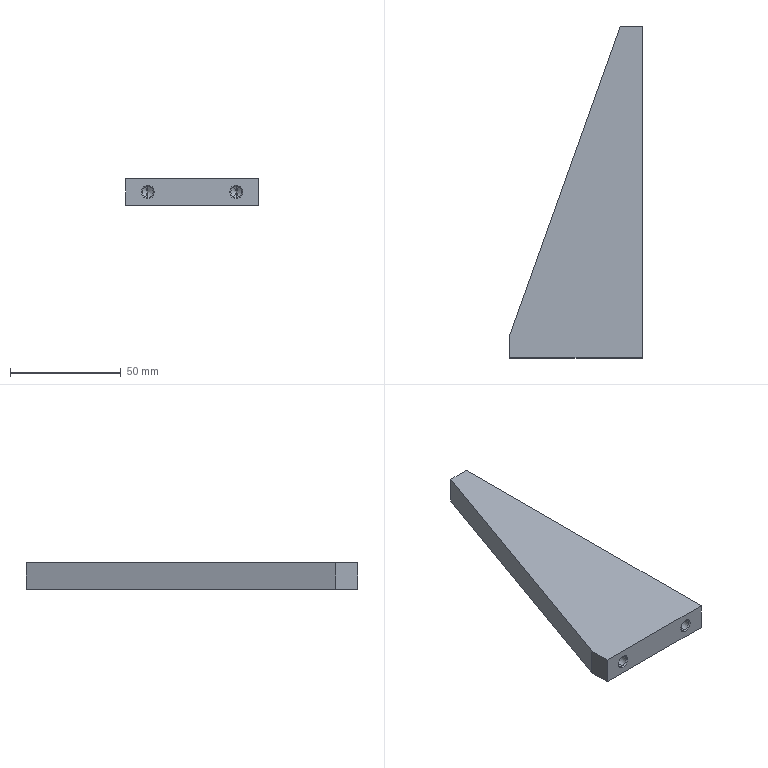Part | SolidWorks | features HoleWzd 2, Extrusion 1 | 1 solid | 31 faces | box 60 x 150 x 12 mm | volume 64773 mm3 | cone 16 | cylinder 8 | plane 7 | commonest cylinder face diameters 5 x8
STEP:
#1=CARTESIAN_POINT('',(59.475,33.456,8.5));
#2=VERTEX_POINT('',#1);
#3=CARTESIAN_POINT('',(59.475,33.456,3.5));
#4=VERTEX_POINT('',#3);
#5=CARTESIAN_POINT('',(59.475,33.456,6.));
#6=DIRECTION('',(1.,0.,0.));
#7=DIRECTION('',(0.,0.,-1.));
#8=AXIS2_PLACEMENT_3D('',#5,#6,#7);
#9=CIRCLE('',#8,2.5);
#10=EDGE_CURVE('',#2,#4,#9,.T.);
#11=ORIENTED_EDGE('',*,*,#10,.F.);
#12=CARTESIAN_POINT('',(60.,33.456,9.025));
#13=VERTEX_POINT('',#12);
#14=CARTESIAN_POINT('',(60.,33.456,9.025));
#15=DIRECTION('',(0.7071,0.,0.7071));
#16=VECTOR('',#15,1000.);
#17=LINE('',#14,#16);
#18=EDGE_CURVE('',#2,#13,#17,.T.);
#19=ORIENTED_EDGE('',*,*,#18,.T.);
#20=CARTESIAN_POINT('',(60.,33.456,2.975));
#21=VERTEX_POINT('',#20);
#22=CARTESIAN_POINT('',(60.,33.456,6.));
#23=DIRECTION('',(1.,0.,0.));
#24=DIRECTION('',(0.,0.,-1.));
#25=AXIS2_PLACEMENT_3D('',#22,#23,#24);
#26=CIRCLE('',#25,3.025);
#27=EDGE_CURVE('',#13,#21,#26,.T.);
#28=ORIENTED_EDGE('',*,*,#27,.T.);
#29=CARTESIAN_POINT('',(60.,33.456,2.975));
#30=DIRECTION('',(0.7071,0.,-0.7071));
#31=VECTOR('',#30,1000.);
#32=LINE('',#29,#31);
#33=EDGE_CURVE('',#4,#21,#32,.T.);
#34=ORIENTED_EDGE('',*,*,#33,.F.);
#35=EDGE_LOOP('',(#11,#19,#28,#34));
#36=FACE_OUTER_BOUND('',#35,.T.);
#37=CARTESIAN_POINT('',(60.,33.456,6.));
#38=DIRECTION('',(1.,0.,0.));
#39=DIRECTION('',(0.,0.,-1.));
#40=AXIS2_PLACEMENT_3D('',#37,#38,#39);
#41=CONICAL_SURFACE('',#40,3.025,0.7854);
#42=ADVANCED_FACE('',(#36),#41,.F.);
#43=CARTESIAN_POINT('',(45.,33.456,8.5));
#44=VERTEX_POINT('',#43);
#45=CARTESIAN_POINT('',(45.,33.456,3.5));
#46=VERTEX_POINT('',#45);
#47=CARTESIAN_POINT('',(45.,33.456,6.));
#48=DIRECTION('',(1.,0.,0.));
#49=DIRECTION('',(0.,0.,-1.));
#50=AXIS2_PLACEMENT_3D('',#47,#48,#49);
#51=CIRCLE('',#50,2.5);
#52=EDGE_CURVE('',#44,#46,#51,.T.);
#53=ORIENTED_EDGE('',*,*,#52,.F.);
#54=CARTESIAN_POINT('',(60.,33.456,8.5));
#55=DIRECTION('',(1.,0.,0.));
#56=VECTOR('',#55,1000.);
#57=LINE('',#54,#56);
#58=EDGE_CURVE('',#44,#2,#57,.T.);
#59=ORIENTED_EDGE('',*,*,#58,.T.);
#60=ORIENTED_EDGE('',*,*,#10,.T.);
#61=CARTESIAN_POINT('',(60.,33.456,3.5));
#62=DIRECTION('',(1.,0.,0.));
#63=VECTOR('',#62,1000.);
#64=LINE('',#61,#63);
#65=EDGE_CURVE('',#46,#4,#64,.T.);
#66=ORIENTED_EDGE('',*,*,#65,.F.);
#67=EDGE_LOOP('',(#53,#59,#60,#66));
#68=FACE_OUTER_BOUND('',#67,.T.);
#69=CARTESIAN_POINT('',(60.,33.456,6.));
#70=DIRECTION('',(1.,0.,0.));
#71=DIRECTION('',(0.,0.,-1.));
#72=AXIS2_PLACEMENT_3D('',#69,#70,#71);
#73=CYLINDRICAL_SURFACE('',#72,2.5);
#74=ADVANCED_FACE('',(#68),#73,.F.);
#75=CARTESIAN_POINT('',(43.498,33.456,6.));
#76=VERTEX_POINT('',#75);
#77=CARTESIAN_POINT('',(45.,33.456,3.5));
#78=DIRECTION('',(0.515,0.,-0.8572));
#79=VECTOR('',#78,1000.);
#80=LINE('',#77,#79);
#81=EDGE_CURVE('',#76,#46,#80,.T.);
#82=ORIENTED_EDGE('',*,*,#81,.F.);
#83=CARTESIAN_POINT('',(45.,33.456,8.5));
#84=DIRECTION('',(0.515,0.,0.8572));
#85=VECTOR('',#84,1000.);
#86=LINE('',#83,#85);
#87=EDGE_CURVE('',#76,#44,#86,.T.);
#88=ORIENTED_EDGE('',*,*,#87,.T.);
#89=ORIENTED_EDGE('',*,*,#52,.T.);
#90=EDGE_LOOP('',(#82,#88,#89));
#91=FACE_OUTER_BOUND('',#90,.T.);
#92=CARTESIAN_POINT('',(45.,33.456,6.));
#93=DIRECTION('',(1.,0.,0.));
#94=DIRECTION('',(0.,0.,-1.));
#95=AXIS2_PLACEMENT_3D('',#92,#93,#94);
#96=CONICAL_SURFACE('',#95,2.5,1.03);
#97=ADVANCED_FACE('',(#91),#96,.F.);
#98=CARTESIAN_POINT('',(59.475,133.456,8.5));
#99=VERTEX_POINT('',#98);
#100=CARTESIAN_POINT('',(59.475,133.456,3.5));
#101=VERTEX_POINT('',#100);
#102=CARTESIAN_POINT('',(59.475,133.456,6.));
#103=DIRECTION('',(1.,0.,0.));
#104=DIRECTION('',(0.,0.,-1.));
#105=AXIS2_PLACEMENT_3D('',#102,#103,#104);
#106=CIRCLE('',#105,2.5);
#107=EDGE_CURVE('',#99,#101,#106,.T.);
#108=ORIENTED_EDGE('',*,*,#107,.F.);
#109=CARTESIAN_POINT('',(60.,133.456,9.025));
#110=VERTEX_POINT('',#109);
#111=CARTESIAN_POINT('',(60.,133.456,9.025));
#112=DIRECTION('',(0.7071,0.,0.7071));
#113=VECTOR('',#112,1000.);
#114=LINE('',#111,#113);
#115=EDGE_CURVE('',#99,#110,#114,.T.);
#116=ORIENTED_EDGE('',*,*,#115,.T.);
#117=CARTESIAN_POINT('',(60.,133.456,2.975));
#118=VERTEX_POINT('',#117);
#119=CARTESIAN_POINT('',(60.,133.456,6.));
#120=DIRECTION('',(1.,0.,0.));
#121=DIRECTION('',(0.,0.,-1.));
#122=AXIS2_PLACEMENT_3D('',#119,#120,#121);
#123=CIRCLE('',#122,3.025);
#124=EDGE_CURVE('',#110,#118,#123,.T.);
#125=ORIENTED_EDGE('',*,*,#124,.T.);
#126=CARTESIAN_POINT('',(60.,133.456,2.975));
#127=DIRECTION('',(0.7071,0.,-0.7071));
#128=VECTOR('',#127,1000.);
#129=LINE('',#126,#128);
#130=EDGE_CURVE('',#101,#118,#129,.T.);
#131=ORIENTED_EDGE('',*,*,#130,.F.);
#132=EDGE_LOOP('',(#108,#116,#125,#131));
#133=FACE_OUTER_BOUND('',#132,.T.);
#134=CARTESIAN_POINT('',(60.,133.456,6.));
#135=DIRECTION('',(1.,0.,0.));
#136=DIRECTION('',(0.,0.,-1.));
#137=AXIS2_PLACEMENT_3D('',#134,#135,#136);
#138=CONICAL_SURFACE('',#137,3.025,0.7854);
#139=ADVANCED_FACE('',(#133),#138,.F.);
#140=CARTESIAN_POINT('',(45.,133.456,8.5));
#141=VERTEX_POINT('',#140);
#142=CARTESIAN_POINT('',(45.,133.456,3.5));
#143=VERTEX_POINT('',#142);
#144=CARTESIAN_POINT('',(45.,133.456,6.));
#145=DIRECTION('',(1.,0.,0.));
#146=DIRECTION('',(0.,0.,-1.));
#147=AXIS2_PLACEMENT_3D('',#144,#145,#146);
#148=CIRCLE('',#147,2.5);
#149=EDGE_CURVE('',#141,#143,#148,.T.);
#150=ORIENTED_EDGE('',*,*,#149,.F.);
#151=CARTESIAN_POINT('',(60.,133.456,8.5));
#152=DIRECTION('',(1.,0.,0.));
#153=VECTOR('',#152,1000.);
#154=LINE('',#151,#153);
#155=EDGE_CURVE('',#141,#99,#154,.T.);
#156=ORIENTED_EDGE('',*,*,#155,.T.);
#157=ORIENTED_EDGE('',*,*,#107,.T.);
#158=CARTESIAN_POINT('',(60.,133.456,3.5));
#159=DIRECTION('',(1.,0.,0.));
#160=VECTOR('',#159,1000.);
#161=LINE('',#158,#160);
#162=EDGE_CURVE('',#143,#101,#161,.T.);
#163=ORIENTED_EDGE('',*,*,#162,.F.);
#164=EDGE_LOOP('',(#150,#156,#157,#163));
#165=FACE_OUTER_BOUND('',#164,.T.);
#166=CARTESIAN_POINT('',(60.,133.456,6.));
#167=DIRECTION('',(1.,0.,0.));
#168=DIRECTION('',(0.,0.,-1.));
#169=AXIS2_PLACEMENT_3D('',#166,#167,#168);
#170=CYLINDRICAL_SURFACE('',#169,2.5);
#171=ADVANCED_FACE('',(#165),#170,.F.);
#172=CARTESIAN_POINT('',(43.498,133.456,6.));
#173=VERTEX_POINT('',#172);
#174=CARTESIAN_POINT('',(45.,133.456,3.5));
#175=DIRECTION('',(0.515,0.,-0.8572));
#176=VECTOR('',#175,1000.);
#177=LINE('',#174,#176);
#178=EDGE_CURVE('',#173,#143,#177,.T.);
#179=ORIENTED_EDGE('',*,*,#178,.F.);
#180=CARTESIAN_POINT('',(45.,133.456,8.5));
#181=DIRECTION('',(0.515,0.,0.8572));
#182=VECTOR('',#181,1000.);
#183=LINE('',#180,#182);
#184=EDGE_CURVE('',#173,#141,#183,.T.);
#185=ORIENTED_EDGE('',*,*,#184,.T.);
#186=ORIENTED_EDGE('',*,*,#149,.T.);
#187=EDGE_LOOP('',(#179,#185,#186));
#188=FACE_OUTER_BOUND('',#187,.T.);
#189=CARTESIAN_POINT('',(45.,133.456,6.));
#190=DIRECTION('',(1.,0.,0.));
#191=DIRECTION('',(0.,0.,-1.));
#192=AXIS2_PLACEMENT_3D('',#189,#190,#191);
#193=CONICAL_SURFACE('',#192,2.5,1.03);
#194=ADVANCED_FACE('',(#188),#193,.F.);
#195=CARTESIAN_POINT('',(50.,8.981,8.5));
#196=VERTEX_POINT('',#195);
#197=CARTESIAN_POINT('',(50.,8.981,3.5));
#198=VERTEX_POINT('',#197);
#199=CARTESIAN_POINT('',(50.,8.981,6.));
#200=DIRECTION('',(0.,-1.,0.));
#201=DIRECTION('',(0.,0.,-1.));
#202=AXIS2_PLACEMENT_3D('',#199,#200,#201);
#203=CIRCLE('',#202,2.5);
#204=EDGE_CURVE('',#196,#198,#203,.T.);
#205=ORIENTED_EDGE('',*,*,#204,.F.);
#206=CARTESIAN_POINT('',(50.,8.456,9.025));
#207=VERTEX_POINT('',#206);
#208=CARTESIAN_POINT('',(50.,8.456,9.025));
#209=DIRECTION('',(0.,-0.7071,0.7071));
#210=VECTOR('',#209,1000.);
#211=LINE('',#208,#210);
#212=EDGE_CURVE('',#196,#207,#211,.T.);
#213=ORIENTED_EDGE('',*,*,#212,.T.);
#214=CARTESIAN_POINT('',(50.,8.456,2.975));
#215=VERTEX_POINT('',#214);
#216=CARTESIAN_POINT('',(50.,8.456,6.));
#217=DIRECTION('',(0.,-1.,0.));
#218=DIRECTION('',(0.,0.,-1.));
#219=AXIS2_PLACEMENT_3D('',#216,#217,#218);
#220=CIRCLE('',#219,3.025);
#221=EDGE_CURVE('',#207,#215,#220,.T.);
#222=ORIENTED_EDGE('',*,*,#221,.T.);
#223=CARTESIAN_POINT('',(50.,8.456,2.975));
#224=DIRECTION('',(0.,-0.7071,-0.7071));
#225=VECTOR('',#224,1000.);
#226=LINE('',#223,#225);
#227=EDGE_CURVE('',#198,#215,#226,.T.);
#228=ORIENTED_EDGE('',*,*,#227,.F.);
#229=EDGE_LOOP('',(#205,#213,#222,#228));
#230=FACE_OUTER_BOUND('',#229,.T.);
#231=CARTESIAN_POINT('',(50.,8.456,6.));
#232=DIRECTION('',(0.,-1.,0.));
#233=DIRECTION('',(0.,0.,-1.));
#234=AXIS2_PLACEMENT_3D('',#231,#232,#233);
#235=CONICAL_SURFACE('',#234,3.025,0.7854);
#236=ADVANCED_FACE('',(#230),#235,.F.);
#237=CARTESIAN_POINT('',(50.,23.456,8.5));
#238=VERTEX_POINT('',#237);
#239=CARTESIAN_POINT('',(50.,23.456,3.5));
#240=VERTEX_POINT('',#239);
#241=CARTESIAN_POINT('',(50.,23.456,6.));
#242=DIRECTION('',(0.,-1.,0.));
#243=DIRECTION('',(0.,0.,-1.));
#244=AXIS2_PLACEMENT_3D('',#241,#242,#243);
#245=CIRCLE('',#244,2.5);
#246=EDGE_CURVE('',#238,#240,#245,.T.);
#247=ORIENTED_EDGE('',*,*,#246,.F.);
#248=CARTESIAN_POINT('',(50.,8.456,8.5));
#249=DIRECTION('',(0.,-1.,0.));
#250=VECTOR('',#249,1000.);
#251=LINE('',#248,#250);
#252=EDGE_CURVE('',#238,#196,#251,.T.);
#253=ORIENTED_EDGE('',*,*,#252,.T.);
#254=ORIENTED_EDGE('',*,*,#204,.T.);
#255=CARTESIAN_POINT('',(50.,8.456,3.5));
#256=DIRECTION('',(0.,-1.,0.));
#257=VECTOR('',#256,1000.);
#258=LINE('',#255,#257);
#259=EDGE_CURVE('',#240,#198,#258,.T.);
#260=ORIENTED_EDGE('',*,*,#259,.F.);
#261=EDGE_LOOP('',(#247,#253,#254,#260));
#262=FACE_OUTER_BOUND('',#261,.T.);
#263=CARTESIAN_POINT('',(50.,8.456,6.));
#264=DIRECTION('',(0.,-1.,0.));
#265=DIRECTION('',(0.,0.,-1.));
#266=AXIS2_PLACEMENT_3D('',#263,#264,#265);
#267=CYLINDRICAL_SURFACE('',#266,2.5);
#268=ADVANCED_FACE('',(#262),#267,.F.);
#269=CARTESIAN_POINT('',(50.,24.959,6.));
#270=VERTEX_POINT('',#269);
#271=CARTESIAN_POINT('',(50.,23.456,3.5));
#272=DIRECTION('',(0.,-0.515,-0.8572));
#273=VECTOR('',#272,1000.);
#274=LINE('',#271,#273);
#275=EDGE_CURVE('',#270,#240,#274,.T.);
#276=ORIENTED_EDGE('',*,*,#275,.F.);
#277=CARTESIAN_POINT('',(50.,23.456,8.5));
#278=DIRECTION('',(0.,-0.515,0.8572));
#279=VECTOR('',#278,1000.);
#280=LINE('',#277,#279);
#281=EDGE_CURVE('',#270,#238,#280,.T.);
#282=ORIENTED_EDGE('',*,*,#281,.T.);
#283=ORIENTED_EDGE('',*,*,#246,.T.);
#284=EDGE_LOOP('',(#276,#282,#283));
#285=FACE_OUTER_BOUND('',#284,.T.);
#286=CARTESIAN_POINT('',(50.,23.456,6.));
#287=DIRECTION('',(0.,-1.,0.));
#288=DIRECTION('',(0.,0.,-1.));
#289=AXIS2_PLACEMENT_3D('',#286,#287,#288);
#290=CONICAL_SURFACE('',#289,2.5,1.03);
#291=ADVANCED_FACE('',(#285),#290,.F.);
#292=CARTESIAN_POINT('',(10.,8.981,8.5));
#293=VERTEX_POINT('',#292);
#294=CARTESIAN_POINT('',(10.,8.981,3.5));
#295=VERTEX_POINT('',#294);
#296=CARTESIAN_POINT('',(10.,8.981,6.));
#297=DIRECTION('',(0.,-1.,0.));
#298=DIRECTION('',(0.,0.,-1.));
#299=AXIS2_PLACEMENT_3D('',#296,#297,#298);
#300=CIRCLE('',#299,2.5);
#301=EDGE_CURVE('',#293,#295,#300,.T.);
#302=ORIENTED_EDGE('',*,*,#301,.F.);
#303=CARTESIAN_POINT('',(10.,8.456,9.025));
#304=VERTEX_POINT('',#303);
#305=CARTESIAN_POINT('',(10.,8.456,9.025));
#306=DIRECTION('',(0.,-0.7071,0.7071));
#307=VECTOR('',#306,1000.);
#308=LINE('',#305,#307);
#309=EDGE_CURVE('',#293,#304,#308,.T.);
#310=ORIENTED_EDGE('',*,*,#309,.T.);
#311=CARTESIAN_POINT('',(10.,8.456,2.975));
#312=VERTEX_POINT('',#311);
#313=CARTESIAN_POINT('',(10.,8.456,6.));
#314=DIRECTION('',(0.,-1.,0.));
#315=DIRECTION('',(0.,0.,-1.));
#316=AXIS2_PLACEMENT_3D('',#313,#314,#315);
#317=CIRCLE('',#316,3.025);
#318=EDGE_CURVE('',#304,#312,#317,.T.);
#319=ORIENTED_EDGE('',*,*,#318,.T.);
#320=CARTESIAN_POINT('',(10.,8.456,2.975));
#321=DIRECTION('',(0.,-0.7071,-0.7071));
#322=VECTOR('',#321,1000.);
#323=LINE('',#320,#322);
#324=EDGE_CURVE('',#295,#312,#323,.T.);
#325=ORIENTED_EDGE('',*,*,#324,.F.);
#326=EDGE_LOOP('',(#302,#310,#319,#325));
#327=FACE_OUTER_BOUND('',#326,.T.);
#328=CARTESIAN_POINT('',(10.,8.456,6.));
#329=DIRECTION('',(0.,-1.,0.));
#330=DIRECTION('',(0.,0.,-1.));
#331=AXIS2_PLACEMENT_3D('',#328,#329,#330);
#332=CONICAL_SURFACE('',#331,3.025,0.7854);
#333=ADVANCED_FACE('',(#327),#332,.F.);
#334=CARTESIAN_POINT('',(10.,23.456,8.5));
#335=VERTEX_POINT('',#334);
#336=CARTESIAN_POINT('',(10.,23.456,3.5));
#337=VERTEX_POINT('',#336);
#338=CARTESIAN_POINT('',(10.,23.456,6.));
#339=DIRECTION('',(0.,-1.,0.));
#340=DIRECTION('',(0.,0.,-1.));
#341=AXIS2_PLACEMENT_3D('',#338,#339,#340);
#342=CIRCLE('',#341,2.5);
#343=EDGE_CURVE('',#335,#337,#342,.T.);
#344=ORIENTED_EDGE('',*,*,#343,.F.);
#345=CARTESIAN_POINT('',(10.,8.456,8.5));
#346=DIRECTION('',(0.,-1.,0.));
#347=VECTOR('',#346,1000.);
#348=LINE('',#345,#347);
#349=EDGE_CURVE('',#335,#293,#348,.T.);
#350=ORIENTED_EDGE('',*,*,#349,.T.);
#351=ORIENTED_EDGE('',*,*,#301,.T.);
#352=CARTESIAN_POINT('',(10.,8.456,3.5));
#353=DIRECTION('',(0.,-1.,0.));
#354=VECTOR('',#353,1000.);
#355=LINE('',#352,#354);
#356=EDGE_CURVE('',#337,#295,#355,.T.);
#357=ORIENTED_EDGE('',*,*,#356,.F.);
#358=EDGE_LOOP('',(#344,#350,#351,#357));
#359=FACE_OUTER_BOUND('',#358,.T.);
#360=CARTESIAN_POINT('',(10.,8.456,6.));
#361=DIRECTION('',(0.,-1.,0.));
#362=DIRECTION('',(0.,0.,-1.));
#363=AXIS2_PLACEMENT_3D('',#360,#361,#362);
#364=CYLINDRICAL_SURFACE('',#363,2.5);
#365=ADVANCED_FACE('',(#359),#364,.F.);
#366=CARTESIAN_POINT('',(10.,24.959,6.));
#367=VERTEX_POINT('',#366);
#368=CARTESIAN_POINT('',(10.,23.456,3.5));
#369=DIRECTION('',(0.,-0.515,-0.8572));
#370=VECTOR('',#369,1000.);
#371=LINE('',#368,#370);
#372=EDGE_CURVE('',#367,#337,#371,.T.);
#373=ORIENTED_EDGE('',*,*,#372,.F.);
#374=CARTESIAN_POINT('',(10.,23.456,8.5));
#375=DIRECTION('',(0.,-0.515,0.8572));
#376=VECTOR('',#375,1000.);
#377=LINE('',#374,#376);
#378=EDGE_CURVE('',#367,#335,#377,.T.);
#379=ORIENTED_EDGE('',*,*,#378,.T.);
#380=ORIENTED_EDGE('',*,*,#343,.T.);
#381=EDGE_LOOP('',(#373,#379,#380));
#382=FACE_OUTER_BOUND('',#381,.T.);
#383=CARTESIAN_POINT('',(10.,23.456,6.));
#384=DIRECTION('',(0.,-1.,0.));
#385=DIRECTION('',(0.,0.,-1.));
#386=AXIS2_PLACEMENT_3D('',#383,#384,#385);
#387=CONICAL_SURFACE('',#386,2.5,1.03);
#388=ADVANCED_FACE('',(#382),#387,.F.);
#389=CARTESIAN_POINT('',(50.,158.456,0.));
#390=VERTEX_POINT('',#389);
#391=CARTESIAN_POINT('',(0.,18.456,0.));
#392=VERTEX_POINT('',#391);
#393=CARTESIAN_POINT('',(0.,18.456,0.));
#394=DIRECTION('',(-0.3363,-0.9417,0.));
#395=VECTOR('',#394,1000.);
#396=LINE('',#393,#395);
#397=EDGE_CURVE('',#390,#392,#396,.T.);
#398=ORIENTED_EDGE('',*,*,#397,.T.);
#399=CARTESIAN_POINT('',(0.,18.456,12.));
#400=VERTEX_POINT('',#399);
#401=CARTESIAN_POINT('',(0.,18.456,12.));
#402=DIRECTION('',(0.,0.,-1.));
#403=VECTOR('',#402,1000.);
#404=LINE('',#401,#403);
#405=EDGE_CURVE('',#400,#392,#404,.T.);
#406=ORIENTED_EDGE('',*,*,#405,.F.);
#407=CARTESIAN_POINT('',(50.,158.456,12.));
#408=VERTEX_POINT('',#407);
#409=CARTESIAN_POINT('',(0.,18.456,12.));
#410=DIRECTION('',(-0.3363,-0.9417,0.));
#411=VECTOR('',#410,1000.);
#412=LINE('',#409,#411);
#413=EDGE_CURVE('',#408,#400,#412,.T.);
#414=ORIENTED_EDGE('',*,*,#413,.F.);
#415=CARTESIAN_POINT('',(50.,158.456,12.));
#416=DIRECTION('',(0.,0.,-1.));
#417=VECTOR('',#416,1000.);
#418=LINE('',#415,#417);
#419=EDGE_CURVE('',#408,#390,#418,.T.);
#420=ORIENTED_EDGE('',*,*,#419,.T.);
#421=EDGE_LOOP('',(#398,#406,#414,#420));
#422=FACE_OUTER_BOUND('',#421,.T.);
#423=CARTESIAN_POINT('',(0.,18.456,12.));
#424=DIRECTION('',(0.9417,-0.3363,0.));
#425=DIRECTION('',(0.3363,0.9417,0.));
#426=AXIS2_PLACEMENT_3D('',#423,#424,#425);
#427=PLANE('',#426);
#428=ADVANCED_FACE('',(#422),#427,.F.);
#429=CARTESIAN_POINT('',(0.,8.456,0.));
#430=VERTEX_POINT('',#429);
#431=CARTESIAN_POINT('',(0.,8.456,0.));
#432=DIRECTION('',(0.,-1.,0.));
#433=VECTOR('',#432,1000.);
#434=LINE('',#431,#433);
#435=EDGE_CURVE('',#392,#430,#434,.T.);
#436=ORIENTED_EDGE('',*,*,#435,.T.);
#437=CARTESIAN_POINT('',(0.,8.456,12.));
#438=VERTEX_POINT('',#437);
#439=CARTESIAN_POINT('',(0.,8.456,12.));
#440=DIRECTION('',(0.,0.,-1.));
#441=VECTOR('',#440,1000.);
#442=LINE('',#439,#441);
#443=EDGE_CURVE('',#438,#430,#442,.T.);
#444=ORIENTED_EDGE('',*,*,#443,.F.);
#445=CARTESIAN_POINT('',(0.,8.456,12.));
#446=DIRECTION('',(0.,-1.,0.));
#447=VECTOR('',#446,1000.);
#448=LINE('',#445,#447);
#449=EDGE_CURVE('',#400,#438,#448,.T.);
#450=ORIENTED_EDGE('',*,*,#449,.F.);
#451=ORIENTED_EDGE('',*,*,#405,.T.);
#452=EDGE_LOOP('',(#436,#444,#450,#451));
#453=FACE_OUTER_BOUND('',#452,.T.);
#454=CARTESIAN_POINT('',(0.,8.456,12.));
#455=DIRECTION('',(1.,0.,0.));
#456=DIRECTION('',(0.,1.,0.));
#457=AXIS2_PLACEMENT_3D('',#454,#455,#456);
#458=PLANE('',#457);
#459=ADVANCED_FACE('',(#453),#458,.F.);
#460=CARTESIAN_POINT('',(50.,8.456,6.));
#461=DIRECTION('',(0.,-1.,0.));
#462=DIRECTION('',(0.,0.,-1.));
#463=AXIS2_PLACEMENT_3D('',#460,#461,#462);
#464=CIRCLE('',#463,3.025);
#465=EDGE_CURVE('',#215,#207,#464,.T.);
#466=ORIENTED_EDGE('',*,*,#465,.F.);
#467=ORIENTED_EDGE('',*,*,#221,.F.);
#468=EDGE_LOOP('',(#466,#467));
#469=FACE_BOUND('',#468,.T.);
#470=CARTESIAN_POINT('',(10.,8.456,6.));
#471=DIRECTION('',(0.,-1.,0.));
#472=DIRECTION('',(0.,0.,-1.));
#473=AXIS2_PLACEMENT_3D('',#470,#471,#472);
#474=CIRCLE('',#473,3.025);
#475=EDGE_CURVE('',#312,#304,#474,.T.);
#476=ORIENTED_EDGE('',*,*,#475,.F.);
#477=ORIENTED_EDGE('',*,*,#318,.F.);
#478=EDGE_LOOP('',(#476,#477));
#479=FACE_BOUND('',#478,.T.);
#480=CARTESIAN_POINT('',(60.,8.456,0.));
#481=VERTEX_POINT('',#480);
#482=CARTESIAN_POINT('',(60.,8.456,0.));
#483=DIRECTION('',(1.,0.,0.));
#484=VECTOR('',#483,1000.);
#485=LINE('',#482,#484);
#486=EDGE_CURVE('',#430,#481,#485,.T.);
#487=ORIENTED_EDGE('',*,*,#486,.T.);
#488=CARTESIAN_POINT('',(60.,8.456,12.));
#489=VERTEX_POINT('',#488);
#490=CARTESIAN_POINT('',(60.,8.456,12.));
#491=DIRECTION('',(0.,0.,-1.));
#492=VECTOR('',#491,1000.);
#493=LINE('',#490,#492);
#494=EDGE_CURVE('',#489,#481,#493,.T.);
#495=ORIENTED_EDGE('',*,*,#494,.F.);
#496=CARTESIAN_POINT('',(60.,8.456,12.));
#497=DIRECTION('',(1.,0.,0.));
#498=VECTOR('',#497,1000.);
#499=LINE('',#496,#498);
#500=EDGE_CURVE('',#438,#489,#499,.T.);
#501=ORIENTED_EDGE('',*,*,#500,.F.);
#502=ORIENTED_EDGE('',*,*,#443,.T.);
#503=EDGE_LOOP('',(#487,#495,#501,#502));
#504=FACE_OUTER_BOUND('',#503,.T.);
#505=CARTESIAN_POINT('',(60.,8.456,12.));
#506=DIRECTION('',(0.,1.,0.));
#507=DIRECTION('',(0.,0.,1.));
#508=AXIS2_PLACEMENT_3D('',#505,#506,#507);
#509=PLANE('',#508);
#510=ADVANCED_FACE('',(#469,#479,#504),#509,.F.);
#511=CARTESIAN_POINT('',(60.,33.456,6.));
#512=DIRECTION('',(1.,0.,0.));
#513=DIRECTION('',(0.,0.,-1.));
#514=AXIS2_PLACEMENT_3D('',#511,#512,#513);
#515=CIRCLE('',#514,3.025);
#516=EDGE_CURVE('',#21,#13,#515,.T.);
#517=ORIENTED_EDGE('',*,*,#516,.F.);
#518=ORIENTED_EDGE('',*,*,#27,.F.);
#519=EDGE_LOOP('',(#517,#518));
#520=FACE_BOUND('',#519,.T.);
#521=CARTESIAN_POINT('',(60.,133.456,6.));
#522=DIRECTION('',(1.,0.,0.));
#523=DIRECTION('',(0.,0.,-1.));
#524=AXIS2_PLACEMENT_3D('',#521,#522,#523);
#525=CIRCLE('',#524,3.025);
#526=EDGE_CURVE('',#118,#110,#525,.T.);
#527=ORIENTED_EDGE('',*,*,#526,.F.);
#528=ORIENTED_EDGE('',*,*,#124,.F.);
#529=EDGE_LOOP('',(#527,#528));
#530=FACE_BOUND('',#529,.T.);
#531=CARTESIAN_POINT('',(60.,158.456,0.));
#532=VERTEX_POINT('',#531);
#533=CARTESIAN_POINT('',(60.,158.456,0.));
#534=DIRECTION('',(0.,1.,0.));
#535=VECTOR('',#534,1000.);
#536=LINE('',#533,#535);
#537=EDGE_CURVE('',#481,#532,#536,.T.);
#538=ORIENTED_EDGE('',*,*,#537,.T.);
#539=CARTESIAN_POINT('',(60.,158.456,12.));
#540=VERTEX_POINT('',#539);
#541=CARTESIAN_POINT('',(60.,158.456,12.));
#542=DIRECTION('',(0.,0.,-1.));
#543=VECTOR('',#542,1000.);
#544=LINE('',#541,#543);
#545=EDGE_CURVE('',#540,#532,#544,.T.);
#546=ORIENTED_EDGE('',*,*,#545,.F.);
#547=CARTESIAN_POINT('',(60.,158.456,12.));
#548=DIRECTION('',(0.,1.,0.));
#549=VECTOR('',#548,1000.);
#550=LINE('',#547,#549);
#551=EDGE_CURVE('',#489,#540,#550,.T.);
#552=ORIENTED_EDGE('',*,*,#551,.F.);
#553=ORIENTED_EDGE('',*,*,#494,.T.);
#554=EDGE_LOOP('',(#538,#546,#552,#553));
#555=FACE_OUTER_BOUND('',#554,.T.);
#556=CARTESIAN_POINT('',(60.,158.456,12.));
#557=DIRECTION('',(-1.,0.,0.));
#558=DIRECTION('',(0.,-1.,0.));
#559=AXIS2_PLACEMENT_3D('',#556,#557,#558);
#560=PLANE('',#559);
#561=ADVANCED_FACE('',(#520,#530,#555),#560,.F.);
#562=CARTESIAN_POINT('',(50.,158.456,0.));
#563=DIRECTION('',(-1.,0.,0.));
#564=VECTOR('',#563,1000.);
#565=LINE('',#562,#564);
#566=EDGE_CURVE('',#532,#390,#565,.T.);
#567=ORIENTED_EDGE('',*,*,#566,.T.);
#568=ORIENTED_EDGE('',*,*,#419,.F.);
#569=CARTESIAN_POINT('',(50.,158.456,12.));
#570=DIRECTION('',(-1.,0.,0.));
#571=VECTOR('',#570,1000.);
#572=LINE('',#569,#571);
#573=EDGE_CURVE('',#540,#408,#572,.T.);
#574=ORIENTED_EDGE('',*,*,#573,.F.);
#575=ORIENTED_EDGE('',*,*,#545,.T.);
#576=EDGE_LOOP('',(#567,#568,#574,#575));
#577=FACE_OUTER_BOUND('',#576,.T.);
#578=CARTESIAN_POINT('',(50.,158.456,12.));
#579=DIRECTION('',(0.,-1.,0.));
#580=DIRECTION('',(0.,0.,-1.));
#581=AXIS2_PLACEMENT_3D('',#578,#579,#580);
#582=PLANE('',#581);
#583=ADVANCED_FACE('',(#577),#582,.F.);
#584=ORIENTED_EDGE('',*,*,#413,.T.);
#585=ORIENTED_EDGE('',*,*,#449,.T.);
#586=ORIENTED_EDGE('',*,*,#500,.T.);
#587=ORIENTED_EDGE('',*,*,#551,.T.);
#588=ORIENTED_EDGE('',*,*,#573,.T.);
#589=EDGE_LOOP('',(#584,#585,#586,#587,#588));
#590=FACE_OUTER_BOUND('',#589,.T.);
#591=CARTESIAN_POINT('',(0.,0.,12.));
#592=DIRECTION('',(0.,0.,-1.));
#593=DIRECTION('',(-1.,0.,0.));
#594=AXIS2_PLACEMENT_3D('',#591,#592,#593);
#595=PLANE('',#594);
#596=ADVANCED_FACE('',(#590),#595,.F.);
#597=ORIENTED_EDGE('',*,*,#397,.F.);
#598=ORIENTED_EDGE('',*,*,#566,.F.);
#599=ORIENTED_EDGE('',*,*,#537,.F.);
#600=ORIENTED_EDGE('',*,*,#486,.F.);
#601=ORIENTED_EDGE('',*,*,#435,.F.);
#602=EDGE_LOOP('',(#597,#598,#599,#600,#601));
#603=FACE_OUTER_BOUND('',#602,.T.);
#604=CARTESIAN_POINT('',(0.,0.,0.));
#605=DIRECTION('',(0.,0.,-1.));
#606=DIRECTION('',(-1.,0.,0.));
#607=AXIS2_PLACEMENT_3D('',#604,#605,#606);
#608=PLANE('',#607);
#609=ADVANCED_FACE('',(#603),#608,.T.);
#610=ORIENTED_EDGE('',*,*,#378,.F.);
#611=ORIENTED_EDGE('',*,*,#372,.T.);
#612=CARTESIAN_POINT('',(10.,23.456,6.));
#613=DIRECTION('',(0.,-1.,0.));
#614=DIRECTION('',(0.,0.,-1.));
#615=AXIS2_PLACEMENT_3D('',#612,#613,#614);
#616=CIRCLE('',#615,2.5);
#617=EDGE_CURVE('',#337,#335,#616,.T.);
#618=ORIENTED_EDGE('',*,*,#617,.T.);
#619=EDGE_LOOP('',(#610,#611,#618));
#620=FACE_OUTER_BOUND('',#619,.T.);
#621=CARTESIAN_POINT('',(10.,23.456,6.));
#622=DIRECTION('',(0.,-1.,0.));
#623=DIRECTION('',(0.,0.,-1.));
#624=AXIS2_PLACEMENT_3D('',#621,#622,#623);
#625=CONICAL_SURFACE('',#624,2.5,1.03);
#626=ADVANCED_FACE('',(#620),#625,.F.);
#627=ORIENTED_EDGE('',*,*,#349,.F.);
#628=ORIENTED_EDGE('',*,*,#617,.F.);
#629=ORIENTED_EDGE('',*,*,#356,.T.);
#630=CARTESIAN_POINT('',(10.,8.981,6.));
#631=DIRECTION('',(0.,-1.,0.));
#632=DIRECTION('',(0.,0.,-1.));
#633=AXIS2_PLACEMENT_3D('',#630,#631,#632);
#634=CIRCLE('',#633,2.5);
#635=EDGE_CURVE('',#295,#293,#634,.T.);
#636=ORIENTED_EDGE('',*,*,#635,.T.);
#637=EDGE_LOOP('',(#627,#628,#629,#636));
#638=FACE_OUTER_BOUND('',#637,.T.);
#639=CARTESIAN_POINT('',(10.,8.456,6.));
#640=DIRECTION('',(0.,-1.,0.));
#641=DIRECTION('',(0.,0.,-1.));
#642=AXIS2_PLACEMENT_3D('',#639,#640,#641);
#643=CYLINDRICAL_SURFACE('',#642,2.5);
#644=ADVANCED_FACE('',(#638),#643,.F.);
#645=ORIENTED_EDGE('',*,*,#309,.F.);
#646=ORIENTED_EDGE('',*,*,#635,.F.);
#647=ORIENTED_EDGE('',*,*,#324,.T.);
#648=ORIENTED_EDGE('',*,*,#475,.T.);
#649=EDGE_LOOP('',(#645,#646,#647,#648));
#650=FACE_OUTER_BOUND('',#649,.T.);
#651=CARTESIAN_POINT('',(10.,8.456,6.));
#652=DIRECTION('',(0.,-1.,0.));
#653=DIRECTION('',(0.,0.,-1.));
#654=AXIS2_PLACEMENT_3D('',#651,#652,#653);
#655=CONICAL_SURFACE('',#654,3.025,0.7854);
#656=ADVANCED_FACE('',(#650),#655,.F.);
#657=ORIENTED_EDGE('',*,*,#281,.F.);
#658=ORIENTED_EDGE('',*,*,#275,.T.);
#659=CARTESIAN_POINT('',(50.,23.456,6.));
#660=DIRECTION('',(0.,-1.,0.));
#661=DIRECTION('',(0.,0.,-1.));
#662=AXIS2_PLACEMENT_3D('',#659,#660,#661);
#663=CIRCLE('',#662,2.5);
#664=EDGE_CURVE('',#240,#238,#663,.T.);
#665=ORIENTED_EDGE('',*,*,#664,.T.);
#666=EDGE_LOOP('',(#657,#658,#665));
#667=FACE_OUTER_BOUND('',#666,.T.);
#668=CARTESIAN_POINT('',(50.,23.456,6.));
#669=DIRECTION('',(0.,-1.,0.));
#670=DIRECTION('',(0.,0.,-1.));
#671=AXIS2_PLACEMENT_3D('',#668,#669,#670);
#672=CONICAL_SURFACE('',#671,2.5,1.03);
#673=ADVANCED_FACE('',(#667),#672,.F.);
#674=ORIENTED_EDGE('',*,*,#252,.F.);
#675=ORIENTED_EDGE('',*,*,#664,.F.);
#676=ORIENTED_EDGE('',*,*,#259,.T.);
#677=CARTESIAN_POINT('',(50.,8.981,6.));
#678=DIRECTION('',(0.,-1.,0.));
#679=DIRECTION('',(0.,0.,-1.));
#680=AXIS2_PLACEMENT_3D('',#677,#678,#679);
#681=CIRCLE('',#680,2.5);
#682=EDGE_CURVE('',#198,#196,#681,.T.);
#683=ORIENTED_EDGE('',*,*,#682,.T.);
#684=EDGE_LOOP('',(#674,#675,#676,#683));
#685=FACE_OUTER_BOUND('',#684,.T.);
#686=CARTESIAN_POINT('',(50.,8.456,6.));
#687=DIRECTION('',(0.,-1.,0.));
#688=DIRECTION('',(0.,0.,-1.));
#689=AXIS2_PLACEMENT_3D('',#686,#687,#688);
#690=CYLINDRICAL_SURFACE('',#689,2.5);
#691=ADVANCED_FACE('',(#685),#690,.F.);
#692=ORIENTED_EDGE('',*,*,#212,.F.);
#693=ORIENTED_EDGE('',*,*,#682,.F.);
#694=ORIENTED_EDGE('',*,*,#227,.T.);
#695=ORIENTED_EDGE('',*,*,#465,.T.);
#696=EDGE_LOOP('',(#692,#693,#694,#695));
#697=FACE_OUTER_BOUND('',#696,.T.);
#698=CARTESIAN_POINT('',(50.,8.456,6.));
#699=DIRECTION('',(0.,-1.,0.));
#700=DIRECTION('',(0.,0.,-1.));
#701=AXIS2_PLACEMENT_3D('',#698,#699,#700);
#702=CONICAL_SURFACE('',#701,3.025,0.7854);
#703=ADVANCED_FACE('',(#697),#702,.F.);
#704=ORIENTED_EDGE('',*,*,#184,.F.);
#705=ORIENTED_EDGE('',*,*,#178,.T.);
#706=CARTESIAN_POINT('',(45.,133.456,6.));
#707=DIRECTION('',(1.,0.,0.));
#708=DIRECTION('',(0.,0.,-1.));
#709=AXIS2_PLACEMENT_3D('',#706,#707,#708);
#710=CIRCLE('',#709,2.5);
#711=EDGE_CURVE('',#143,#141,#710,.T.);
#712=ORIENTED_EDGE('',*,*,#711,.T.);
#713=EDGE_LOOP('',(#704,#705,#712));
#714=FACE_OUTER_BOUND('',#713,.T.);
#715=CARTESIAN_POINT('',(45.,133.456,6.));
#716=DIRECTION('',(1.,0.,0.));
#717=DIRECTION('',(0.,0.,-1.));
#718=AXIS2_PLACEMENT_3D('',#715,#716,#717);
#719=CONICAL_SURFACE('',#718,2.5,1.03);
#720=ADVANCED_FACE('',(#714),#719,.F.);
#721=ORIENTED_EDGE('',*,*,#155,.F.);
#722=ORIENTED_EDGE('',*,*,#711,.F.);
#723=ORIENTED_EDGE('',*,*,#162,.T.);
#724=CARTESIAN_POINT('',(59.475,133.456,6.));
#725=DIRECTION('',(1.,0.,0.));
#726=DIRECTION('',(0.,0.,-1.));
#727=AXIS2_PLACEMENT_3D('',#724,#725,#726);
#728=CIRCLE('',#727,2.5);
#729=EDGE_CURVE('',#101,#99,#728,.T.);
#730=ORIENTED_EDGE('',*,*,#729,.T.);
#731=EDGE_LOOP('',(#721,#722,#723,#730));
#732=FACE_OUTER_BOUND('',#731,.T.);
#733=CARTESIAN_POINT('',(60.,133.456,6.));
#734=DIRECTION('',(1.,0.,0.));
#735=DIRECTION('',(0.,0.,-1.));
#736=AXIS2_PLACEMENT_3D('',#733,#734,#735);
#737=CYLINDRICAL_SURFACE('',#736,2.5);
#738=ADVANCED_FACE('',(#732),#737,.F.);
#739=ORIENTED_EDGE('',*,*,#115,.F.);
#740=ORIENTED_EDGE('',*,*,#729,.F.);
#741=ORIENTED_EDGE('',*,*,#130,.T.);
#742=ORIENTED_EDGE('',*,*,#526,.T.);
#743=EDGE_LOOP('',(#739,#740,#741,#742));
#744=FACE_OUTER_BOUND('',#743,.T.);
#745=CARTESIAN_POINT('',(60.,133.456,6.));
#746=DIRECTION('',(1.,0.,0.));
#747=DIRECTION('',(0.,0.,-1.));
#748=AXIS2_PLACEMENT_3D('',#745,#746,#747);
#749=CONICAL_SURFACE('',#748,3.025,0.7854);
#750=ADVANCED_FACE('',(#744),#749,.F.);
#751=ORIENTED_EDGE('',*,*,#87,.F.);
#752=ORIENTED_EDGE('',*,*,#81,.T.);
#753=CARTESIAN_POINT('',(45.,33.456,6.));
#754=DIRECTION('',(1.,0.,0.));
#755=DIRECTION('',(0.,0.,-1.));
#756=AXIS2_PLACEMENT_3D('',#753,#754,#755);
#757=CIRCLE('',#756,2.5);
#758=EDGE_CURVE('',#46,#44,#757,.T.);
#759=ORIENTED_EDGE('',*,*,#758,.T.);
#760=EDGE_LOOP('',(#751,#752,#759));
#761=FACE_OUTER_BOUND('',#760,.T.);
#762=CARTESIAN_POINT('',(45.,33.456,6.));
#763=DIRECTION('',(1.,0.,0.));
#764=DIRECTION('',(0.,0.,-1.));
#765=AXIS2_PLACEMENT_3D('',#762,#763,#764);
#766=CONICAL_SURFACE('',#765,2.5,1.03);
#767=ADVANCED_FACE('',(#761),#766,.F.);
#768=ORIENTED_EDGE('',*,*,#58,.F.);
#769=ORIENTED_EDGE('',*,*,#758,.F.);
#770=ORIENTED_EDGE('',*,*,#65,.T.);
#771=CARTESIAN_POINT('',(59.475,33.456,6.));
#772=DIRECTION('',(1.,0.,0.));
#773=DIRECTION('',(0.,0.,-1.));
#774=AXIS2_PLACEMENT_3D('',#771,#772,#773);
#775=CIRCLE('',#774,2.5);
#776=EDGE_CURVE('',#4,#2,#775,.T.);
#777=ORIENTED_EDGE('',*,*,#776,.T.);
#778=EDGE_LOOP('',(#768,#769,#770,#777));
#779=FACE_OUTER_BOUND('',#778,.T.);
#780=CARTESIAN_POINT('',(60.,33.456,6.));
#781=DIRECTION('',(1.,0.,0.));
#782=DIRECTION('',(0.,0.,-1.));
#783=AXIS2_PLACEMENT_3D('',#780,#781,#782);
#784=CYLINDRICAL_SURFACE('',#783,2.5);
#785=ADVANCED_FACE('',(#779),#784,.F.);
#786=ORIENTED_EDGE('',*,*,#18,.F.);
#787=ORIENTED_EDGE('',*,*,#776,.F.);
#788=ORIENTED_EDGE('',*,*,#33,.T.);
#789=ORIENTED_EDGE('',*,*,#516,.T.);
#790=EDGE_LOOP('',(#786,#787,#788,#789));
#791=FACE_OUTER_BOUND('',#790,.T.);
#792=CARTESIAN_POINT('',(60.,33.456,6.));
#793=DIRECTION('',(1.,0.,0.));
#794=DIRECTION('',(0.,0.,-1.));
#795=AXIS2_PLACEMENT_3D('',#792,#793,#794);
#796=CONICAL_SURFACE('',#795,3.025,0.7854);
#797=ADVANCED_FACE('',(#791),#796,.F.);
#798=CLOSED_SHELL('',(#42,#74,#97,#139,#171,#194,#236,#268,#291,#333,#365,#388,#428,#459,#510,#561,#583,#596,#609,#626,#644,#656,#673,#691,#703,#720,#738,#750,#767,#785,#797));
#799=MANIFOLD_SOLID_BREP('',#798);
#800=CARTESIAN_POINT('',(0.,0.,0.));
#801=DIRECTION('',(0.,0.,1.));
#802=DIRECTION('',(1.,0.,0.));
#803=AXIS2_PLACEMENT_3D('',#800,#801,#802);
#804=(LENGTH_UNIT()NAMED_UNIT(*)SI_UNIT(.MILLI.,.METRE.));
#805=UNCERTAINTY_MEASURE_WITH_UNIT(LENGTH_MEASURE(0.00001),#804,'','');
#806=(NAMED_UNIT(*)PLANE_ANGLE_UNIT()SI_UNIT($,.RADIAN.));
#807=(NAMED_UNIT(*)SI_UNIT($,.STERADIAN.)SOLID_ANGLE_UNIT());
#808=(GEOMETRIC_REPRESENTATION_CONTEXT(3)GLOBAL_UNCERTAINTY_ASSIGNED_CONTEXT((#805))GLOBAL_UNIT_ASSIGNED_CONTEXT((#804,#806,#807))REPRESENTATION_CONTEXT('',''));
#809=ADVANCED_BREP_SHAPE_REPRESENTATION('',(#799,#803),#808);